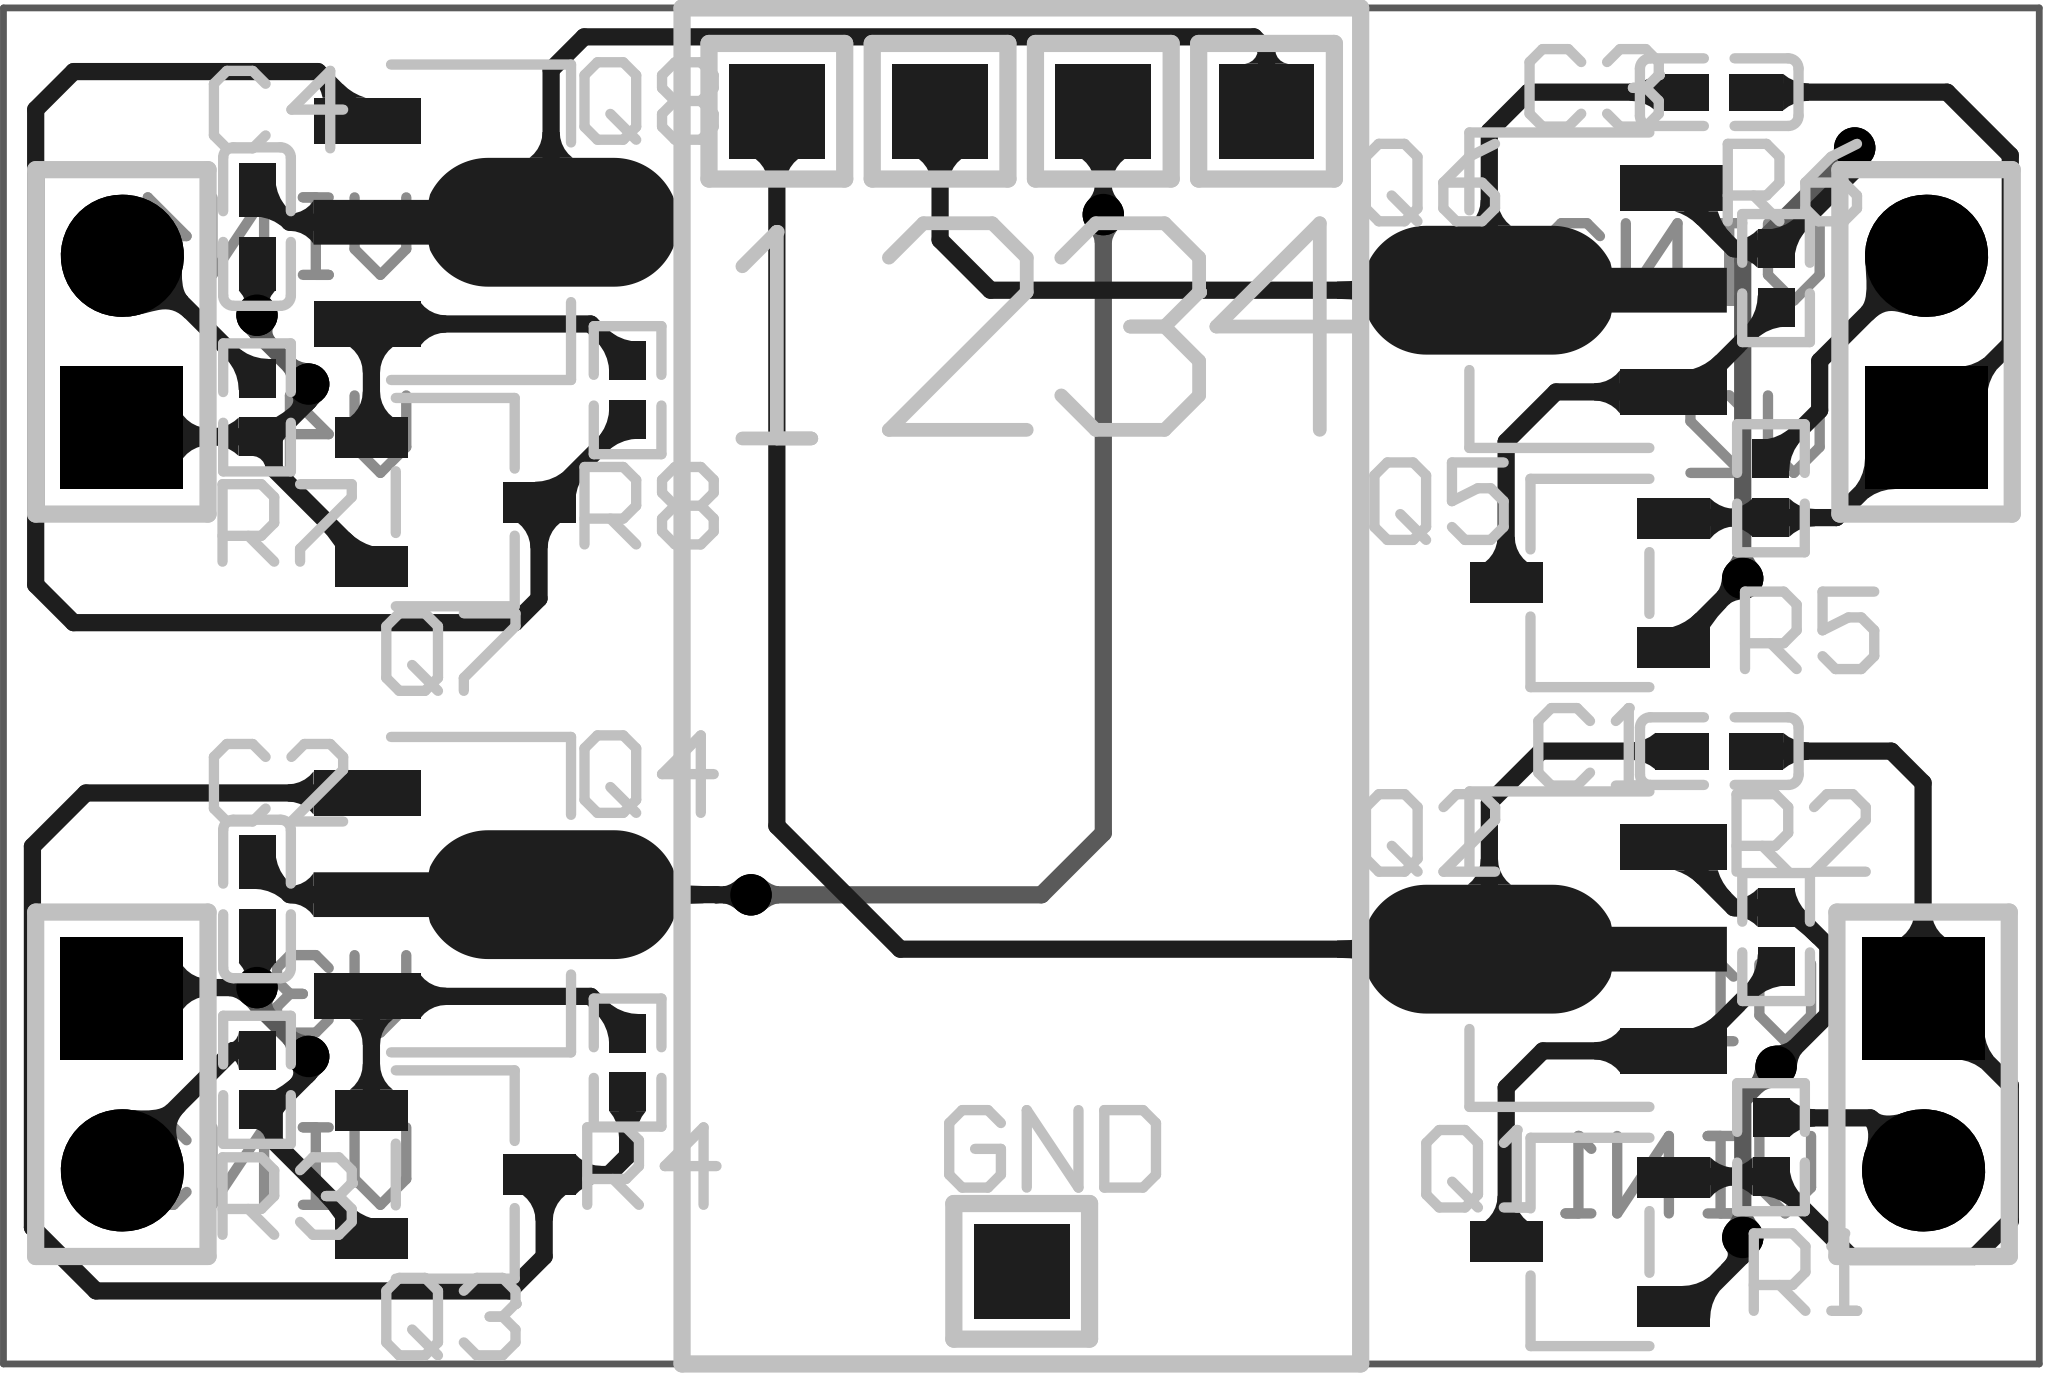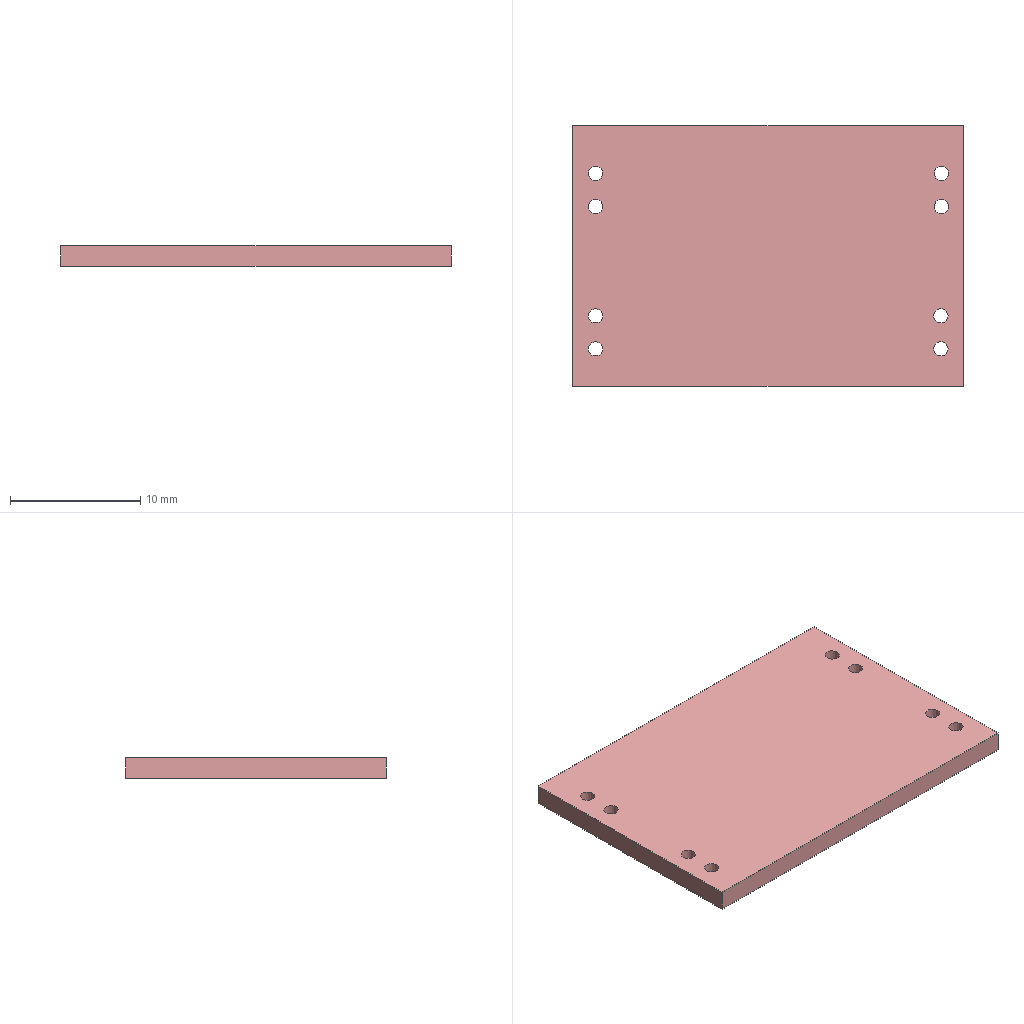Circuit board layout | Altium Designer | box 30 x 20 x 1.6 mm
Layer stack:
# Altium Designer layer stack of  (unit mm; dielectric type: 0 none, 1 core, 2 prepreg, 3 surface material)
index,name,kind,layer,copper_thickness_mm,dielectric_type,dielectric_thickness_mm,dielectric_material,dielectric_constant
0,Top Paste Mask Layer,other,,,,,,
1,Top Silkscreen Layer,other,,,,,,
2,Top Solder Mask Layer,dielectric,,,3,0.01,,3.3
3,Top Layer,copper,Top Layer,0.035,,,,
4,Dielectric1,dielectric,,,3,1.51,FR4,4.5
5,Bottom Layer,copper,Bottom Layer,0.035,,,,
6,Bottom Solder Mask Layer,dielectric,,,3,0.01,,3.3
7,Bottom Silkscreen Layer,other,,,,,,
8,Bottom Paste Mask Layer,other,,,,,,
# drill layer pairs: low layer,high layer
drill_pair,Top Layer,Bottom Layer
Part placement:
Designator,Comment,Layer,Footprint,Center-X(mm),Center-Y(mm),Rotation
H6,,TopLayer,HDR-TH_1P-V-M_XKB_X4611WV-01I-C28D40,87.597,94.676,0
H7,,TopLayer,HDR-TH_1P-V-M_XKB_X4611WV-01I-C28D40,90.002,94.676,0
H8,,TopLayer,HDR-TH_1P-V-M_XKB_X4611WV-01I-C28D40,92.408,94.676,0
H9,,TopLayer,HDR-TH_1P-V-M_XKB_X4611WV-01I-C28D40,94.813,94.676,0
H1,,TopLayer,HDR-TH_2P-P2.54-V-M-1,104.488,80.325,270
H3,,TopLayer,HDR-TH_2P-P2.54-V-M-1,77.945,80.325,270
H4,,TopLayer,HDR-TH_2P-P2.54-V-M-1,77.945,91.275,90
C1,1nF,TopLayer,C0402,101.485,85.239,0
C2,1nF,TopLayer,C0402,79.936,83.058,270
C3,1nF,TopLayer,C0402,101.484,94.957,0
C4,1nF,TopLayer,C0402,79.936,92.975,270
Q1,BC856B,TopLayer,SOT-23-3_L2.9-W1.6-P1.90-LS2.8-BR,99.58,78,0
Q2,2N2222AU,TopLayer,SOT-89-3_L4.5-W2.4-P1.50-LS4.0-BR,99.648,82.318,0
Q3,BC856B,TopLayer,SOT-23-3_L2.9-W1.6-P1.90-LS2.8-BR,82.858,78.994,180
Q4,2N2222AU,TopLayer,SOT-89-3_L4.5-W2.4-P1.50-LS4.0-BR,82.719,83.121,180
Q5,BC856B,TopLayer,SOT-23-3_L2.9-W1.6-P1.90-LS2.8-BR,99.579,87.719,0
Q6,2N2222AU,TopLayer,SOT-89-3_L4.5-W2.4-P1.50-LS4.0-BR,99.647,92.037,0
Q7,BC856B,TopLayer,SOT-23-3_L2.9-W1.6-P1.90-LS2.8-BR,82.858,88.911,180
Q8,2N2222AU,TopLayer,SOT-89-3_L4.5-W2.4-P1.50-LS4.0-BR,82.719,93.038,180
R1,3.9K,TopLayer,R0402,102.247,79.397,270
R2,200k,TopLayer,R0402,102.322,82.496,90
R3,3.9K,TopLayer,R0402,79.936,80.391,270
R4,200k,TopLayer,R0402,85.397,80.645,90
R5,3.9K,TopLayer,R0402,102.246,89.115,270
R6,200k,TopLayer,R0402,102.321,92.215,90
R7,3.9K,TopLayer,R0402,79.936,90.308,270
R8,200k,TopLayer,R0402,85.397,90.562,90
H5,,TopLayer,HDR-TH_2P-P2.54-V-M-1,104.532,91.275,90
H10,,TopLayer,HDR-TH_1P-V-M_XKB_X4611WV-01I-C28D40,91.205,77.566,0
Pad and via stacks:
# Altium Designer via and pad stacks of  (unit mm). Each distinct definition once, with the count of objects using it.
# via: kind,start_layer,end_layer,hole_mm,diameter_mm,mode(0 simple;1 top-mid-bottom;2 full stack),diameter_per_layer,count,example_net
# pad: kind,layer,hole_mm,hole_type(0 round;1 square;2 slot),plating,top_size,top_shape(1 round;2 rect;3 octagon;9 rounded rect),mid_size,bottom_size,mode,footprint,size_per_layer,count,example
pad,Top Layer,0,0,plated,1.4x1.4,2,1.4x1.4,1.4x1.4,0,HDR-TH_1P-V-M_XKB_X4611WV-01I-C28D40,,5,H6.1
pad,Top Layer,0,0,plated,0.7901x0.54,2,0.7901x0.54,0.7901x0.54,0,C0402,,8,C1.2
pad,Top Layer,0,0,plated,1.07x0.6,2,1.07x0.6,1.07x0.6,0,SOT-23-3_L2.9-W1.6-P1.90-LS2.8-BR,,12,Q1.1
pad,Top Layer,0,0,plated,0.95x0.95,1,0.95x0.95,0.95x0.95,0,SOT-89-3_L4.5-W2.4-P1.50-LS4.0-BR,,4,Q2.2
pad,Top Layer,0,0,plated,1.575x0.672,2,1.575x0.672,1.575x0.672,0,SOT-89-3_L4.5-W2.4-P1.50-LS4.0-BR,,8,Q2.3
pad,Top Layer,0,0,plated,0.5657x0.54,2,0.5657x0.54,0.5657x0.54,0,R0402,,16,R1.2
pad,Multi-Layer,1.1,0,plated,1.8x1.8,1,1.8x1.8,1.8x1.8,0,HDR-TH_2P-P2.54-V-M-1,,4,H1.2
pad,Multi-Layer,1.1,0,plated,1.8x1.8,2,1.8x1.8,1.8x1.8,0,HDR-TH_2P-P2.54-V-M-1,,4,H1.1
via,Top Layer,Bottom Layer,0.3048,0.61,0,,10,$1N1514